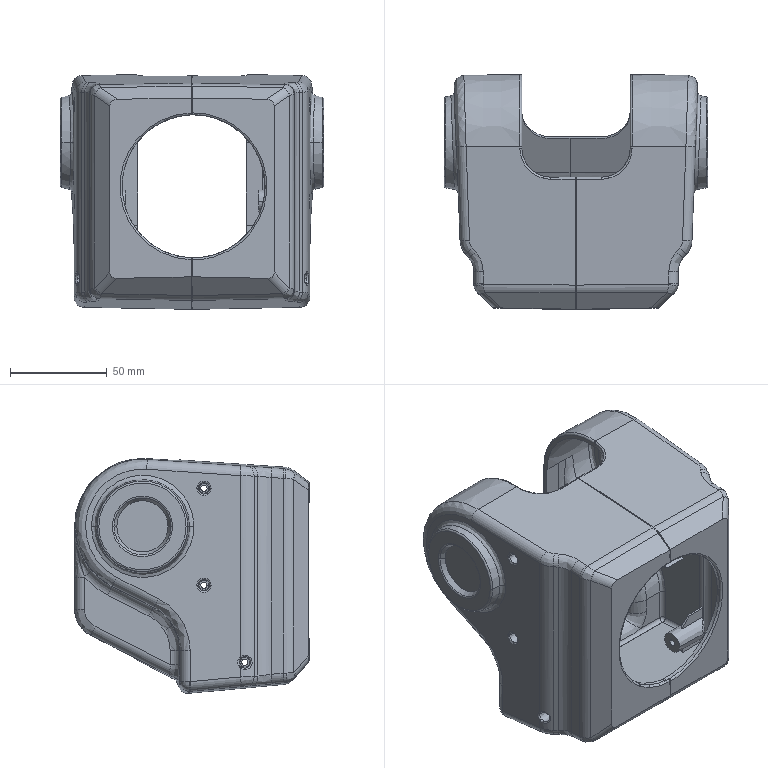Part | NX | features BREP 6 | 6 solids | 541 faces | box 136.184 x 121.469 x 121.428 mm | volume 181259 mm3 | plane 165 | cylinder 158 | spline 155 | cone 40 | torus 15 | sphere 8 | commonest cylinder face diameters 10 x28 4 x26 2 x13 3.2 x12 31.155 x8 45.148 x8